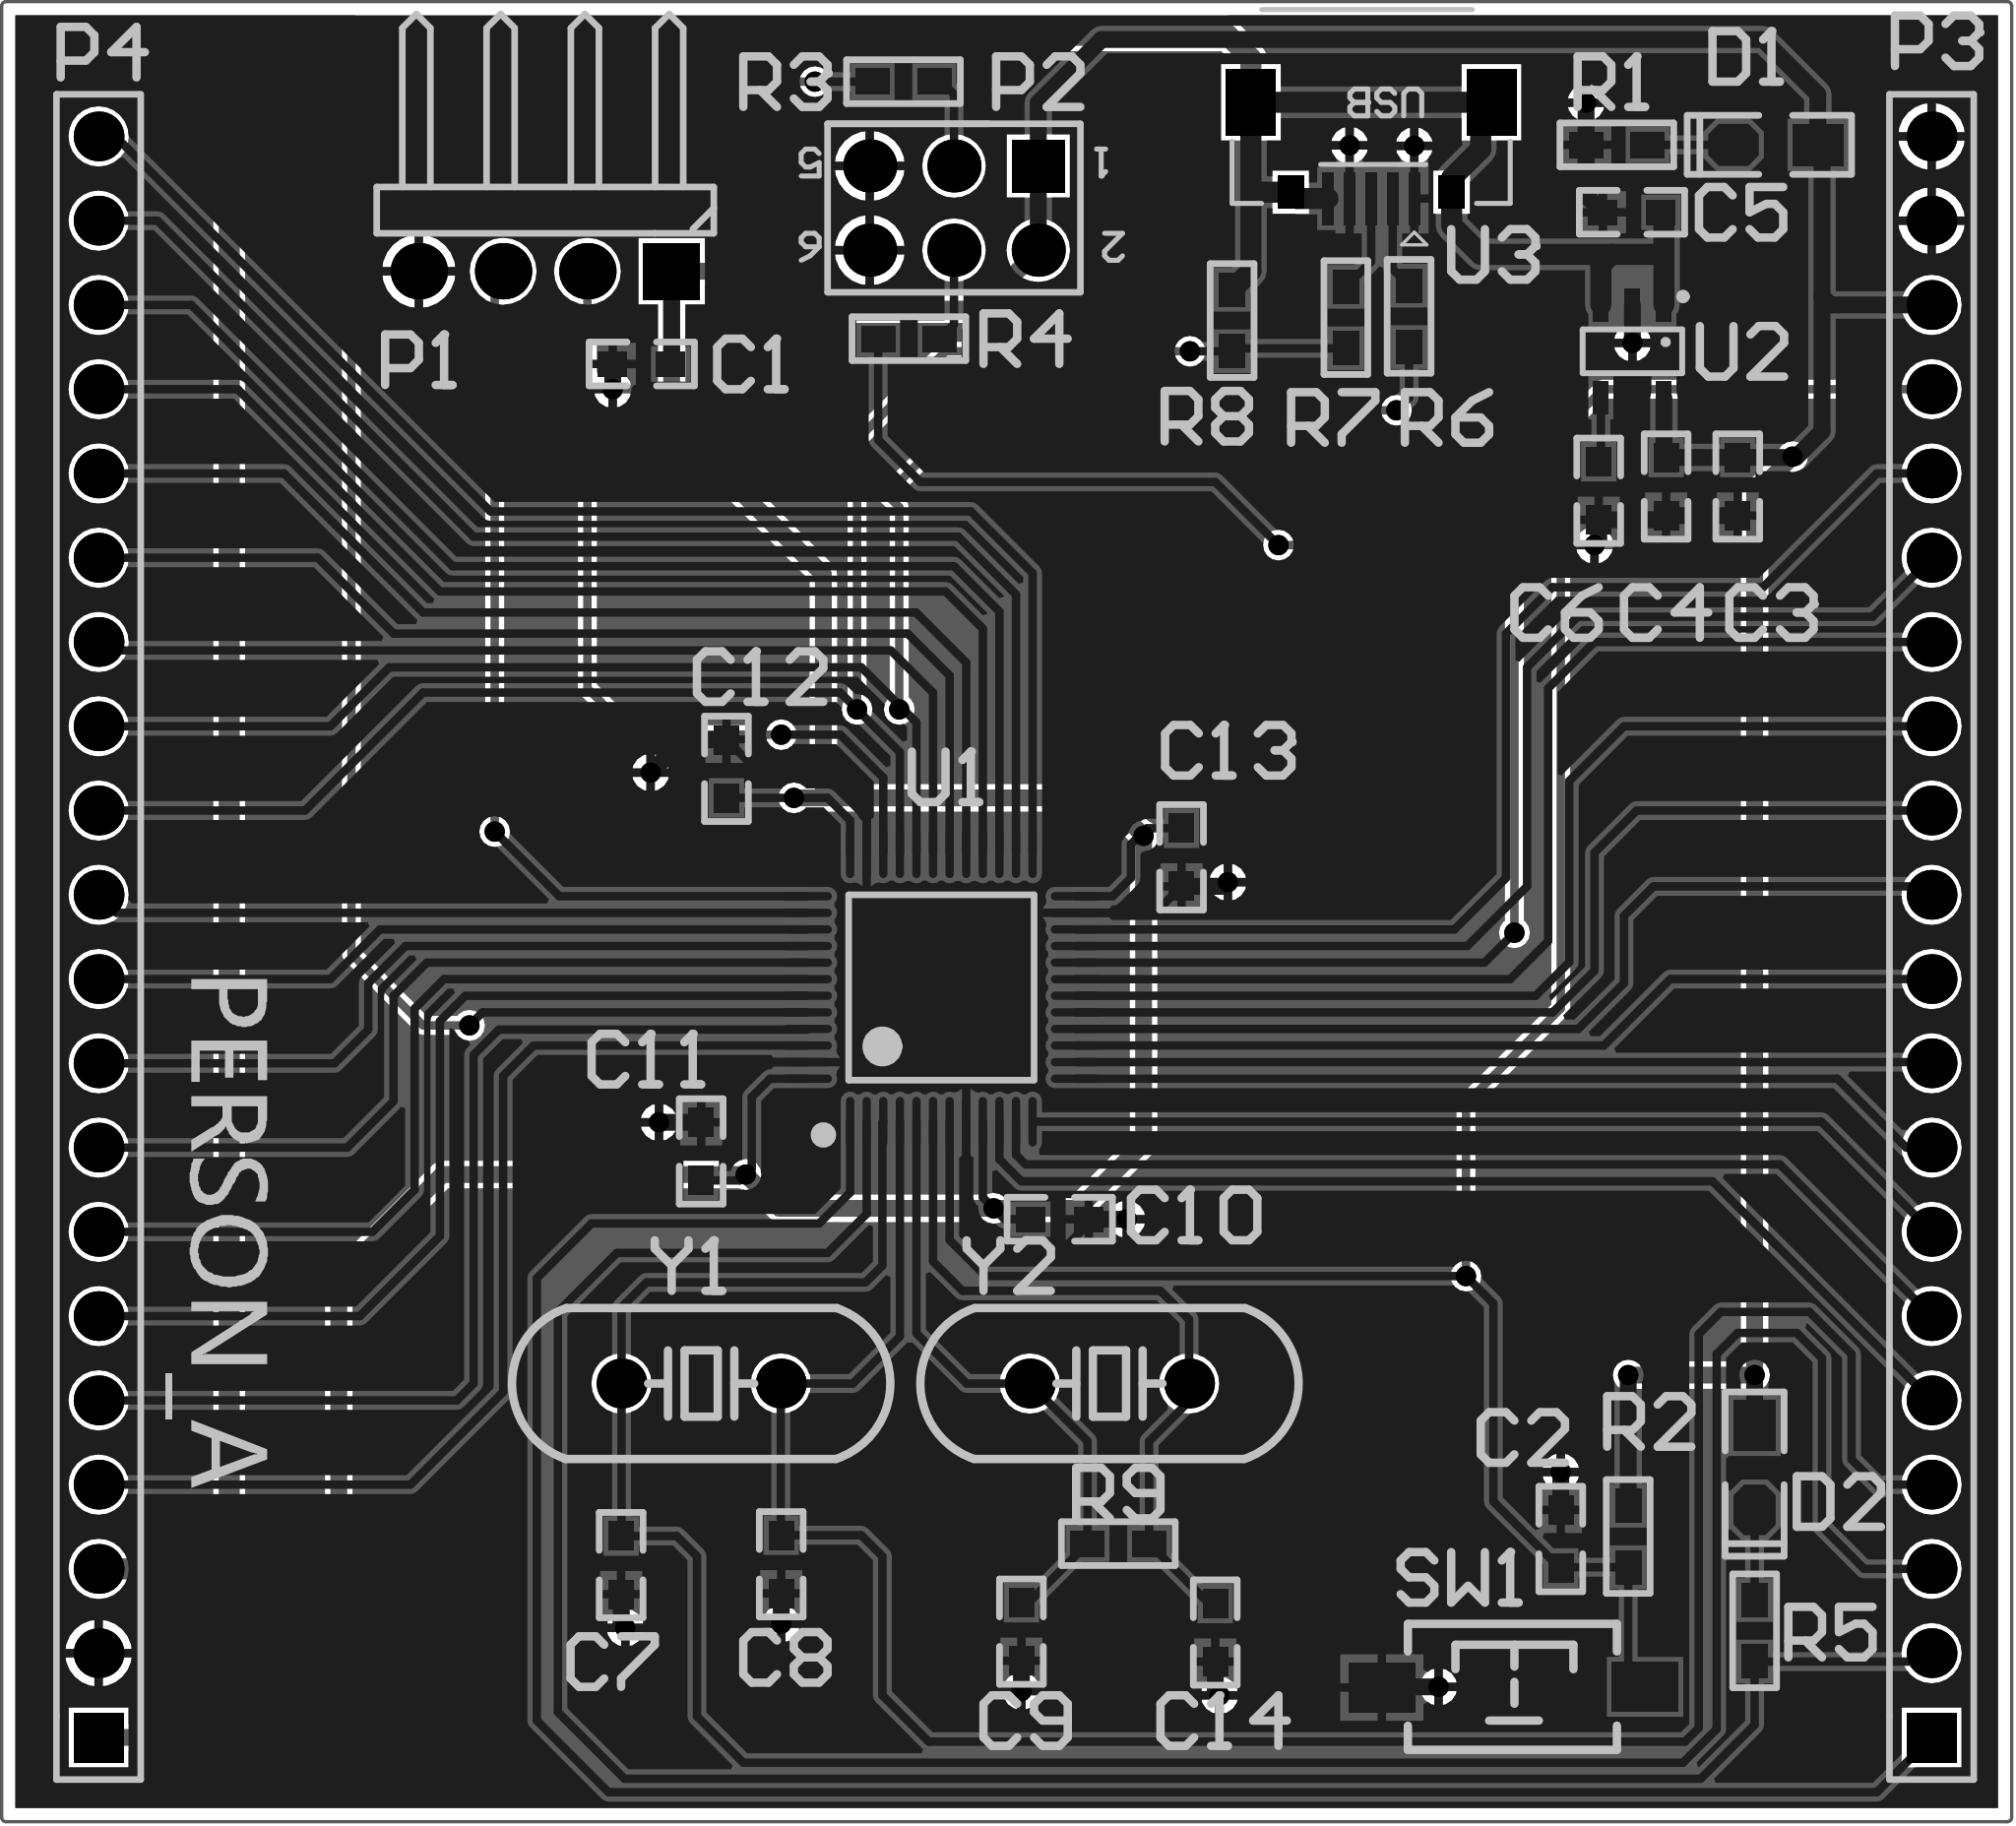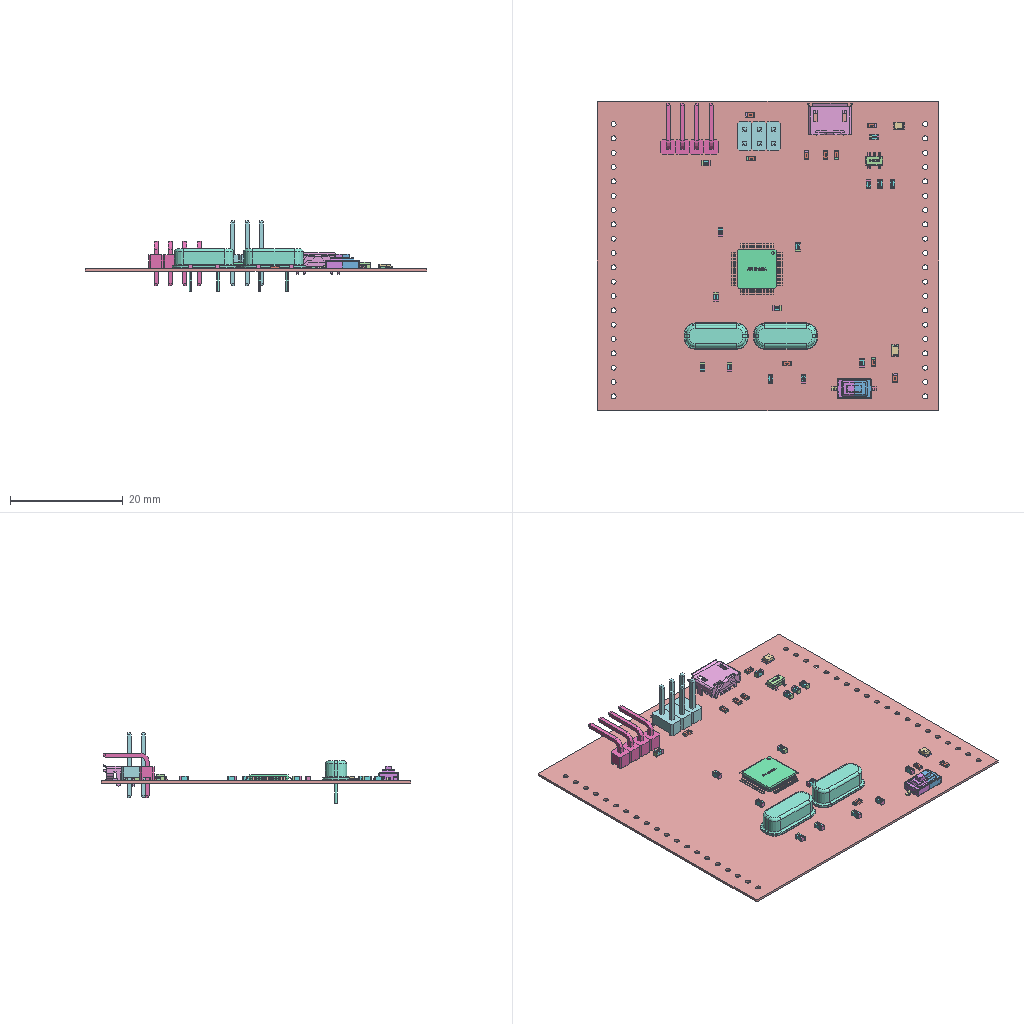Circuit board layout | Altium Designer | box 60.6 x 54.9 x 12.5 mm
Layer stack:
# Altium Designer layer stack of  (unit mm; dielectric type: 0 none, 1 core, 2 prepreg, 3 surface material)
index,name,kind,layer,copper_thickness_mm,dielectric_type,dielectric_thickness_mm,dielectric_material,dielectric_constant
0,Top Paste,other,,,,,,
1,Top Overlay,other,,,,,,
2,Top Solder,dielectric,,,3,0.0102,Solder Resist,3.5
3,Top Layer,copper,Top Layer,0.0356,,,,
4,Dielectric 1,dielectric,,,0,0.32,FR-4,4.8
5,Bottom Layer,copper,Bottom Layer,0.0356,,,,
6,Bottom Solder,dielectric,,,3,0.0102,Solder Resist,3.5
7,Bottom Overlay,other,,,,,,
8,Bottom Paste,other,,,,,,
# drill layer pairs: low layer,high layer
drill_pair,Top Layer,Bottom Layer
Part placement:
Designator,Comment,Layer,Footprint,Center-X(mm),Center-Y(mm),Rotation
C1,105 C0603,TopLayer,C_0603,84.569,116.205,0
C2,105 C0603,TopLayer,C_0603,112.268,80.785,270
C3,105 C0603,TopLayer,C_0603,117.602,112.509,90
C4,105 C0603,TopLayer,C_0603,115.443,112.509,90
C5,105 C0603,TopLayer,C_0603,114.414,120.777,0
C6,105 C0603,TopLayer,C_0603,113.411,112.382,90
C7,22P,0603,TopLayer,C_0603,83.947,79.997,270
C8,22P,0603,TopLayer,C_0603,88.773,80.023,270
C9,22P,0603,TopLayer,C_0603,96.012,77.991,270
C10,105 C0603,TopLayer,C_0603,97.168,90.424,180
C11,105 C0603,TopLayer,C_0603,86.36,92.469,270
C12,105 C0603,TopLayer,C_0603,87.122,104,270
C13,105 C0603,TopLayer,C_0603,100.838,101.333,90
C14,22P,0603,TopLayer,C_0603,101.854,77.965,270
D1,LED,TopLayer,LED_0805G,118.745,122.809,180
D2,LED,TopLayer,LED_0805G,118.11,82.931,270
P1,SWD,TopLayer,HDR-1X4_H,81.661,118.999,180
P2,Header 3X2,TopLayer,HDR-3X2,93.98,120.904,180
P3,Header 20,TopLayer,HDR1X20,123.444,98.933,90
P4,Header 20,TopLayer,HDR1X20,68.199,98.933,90
R1,10K R0603,TopLayer,R_0603,113.957,122.809,180
R3,10K R0603,TopLayer,R_0603,92.456,124.714,0
R4,10K R0603,TopLayer,R_0603,92.621,116.967,180
R5,10K R0603,TopLayer,R_0603,118.11,78.016,270
R6,20R,0603,TopLayer,R_0603,107.696,117.64,270
R7,20R0603,TopLayer,R_0603,105.791,117.602,270
R8,4.7K,0603,TopLayer,R_0603,102.362,117.513,270
R9,1M0603,TopLayer,R_0603,98.933,80.645,180
SW1,SW-PB_V,TopLayer,TSW_SMD-3*6*2.5,110.842,76.317,360
U1,stm32f103c8t6_48pin,TopLayer,TQFP48_7x7_L,93.599,97.409,0
U2,RT9193,TopLayer,SOT23-5L,114.427,116.586,180
U3,USB-mrico,TopLayer,USB-micro_B,106.553,122.642,180
Y1,32.768K,TopLayer,XTAL-49S_DIP,86.36,85.471,180
Y2,8M,TopLayer,XTAL-49S_DIP,98.666,85.471,180
R2,10K R0603,TopLayer,R_0603,114.3,80.861,90
Pad and via stacks:
# Altium Designer via and pad stacks of  (unit mm). Each distinct definition once, with the count of objects using it.
# via: kind,start_layer,end_layer,hole_mm,diameter_mm,mode(0 simple;1 top-mid-bottom;2 full stack),diameter_per_layer,count,example_net
# pad: kind,layer,hole_mm,hole_type(0 round;1 square;2 slot),plating,top_size,top_shape(1 round;2 rect;3 octagon;9 rounded rect),mid_size,bottom_size,mode,footprint,size_per_layer,count,example
pad,Top Layer,0,0,plated,0.889x0.762,2,0.889x0.762,0.889x0.762,0,C 0603,,28,C14.2
pad,Top Layer,0,0,plated,1.016x0.8,2,1.016x0.8,1.016x0.8,0,R 0603,,18,R9.1
pad,Top Layer,0,0,plated,1.6x0.35,2,1.6x0.35,1.6x0.35,0,USB-micro_B,,5,U3.2
pad,Top Layer,0,0,plated,0.45x1,2,0.45x1,0.45x1,0,SOT23-5L,,5,U2.4
pad,Top Layer,0,0,plated,0.25x1.5,1,0.25x1.5,0.25x1.5,0,TQFP48 7x7_L,,48,U1.1
pad,Top Layer,0,0,plated,2x1.5,2,2x1.5,2x1.5,0,TSW SMD-3*6*2.5,,2,SW1.1
pad,Top Layer,0,0,plated,1.524x1.27,2,1.524x1.27,1.524x1.27,0,LED 0805G,,2,D2.1
pad,Top Layer,0,0,plated,1.524x1.27,3,1.524x1.27,1.524x1.27,0,LED 0805G,,2,D2.2
pad,Multi-Layer,0.8,0,plated,1.5x1.5,1,1.5x1.5,1.5x1.5,0,XTAL-49S DIP,,4,Y2.2
pad,Multi-Layer,0.5,2,plated,1.5x2,2,1.5x2,1.5x2,0,USB-micro_B,,2,U3.5
pad,Multi-Layer,0.5,0,plated,0.8x1,2,0.8x1,0.8x1,0,USB-micro_B,,2,U3.5
pad,Multi-Layer,0.9,0,plated,1.5x1.5,2,1.5x1.5,1.5x1.5,0,HDR1X20,,2,P4.1
pad,Multi-Layer,0.9,0,plated,1.5x1.5,1,1.5x1.5,1.5x1.5,0,HDR1X20,,38,P4.2
pad,Multi-Layer,0.9,0,plated,1.6x1.6,2,1.6x1.6,1.6x1.6,0,HDR-3X2,,1,P2.1
pad,Multi-Layer,0.9,0,plated,1.6x1.6,1,1.6x1.6,1.6x1.6,0,HDR-3X2,,5,P2.2
pad,Multi-Layer,0.9,0,plated,1.7x1.7,2,1.7x1.7,1.7x1.7,0,HDR-1X4_H,,1,P1.1
pad,Multi-Layer,0.9,0,plated,1.7x1.7,1,1.7x1.7,1.7x1.7,0,HDR-1X4_H,,3,P1.2
via,Top Layer,Bottom Layer,0.3048,0.6096,0,,34,SWDCLK
Copper pours:
name,layer,net,type(0 solid;1 hatched;2 none)
D,Top Layer,GND,0
D,Bottom Layer,GND,0
Design rules, without the lines most boards share:
# Altium Designer design rules of  (exported by Altium Designer, unit mm)
# columns: name | kind | enabled | priority | scope1 | scope2 | descriptor | typed fields (field=value)
Clearance | 0 | enabled | 1 | All | All | Clearance Constraint (Gap=6mil) (All),(All) | gap=0.1524
PlaneConnect | 6 | enabled | 1 | All | All | Power Plane Connect Rule(Relief Connect )(Expansion=20mil) (Conductor Width=10mil) (Air Gap=10mil) (Entries=4) (All) | relief_conductor_width=0.254 relief_entries=4 relief_expansion=0.508
PolygonConnect | 20 | enabled | 1 | All | All | Polygon Connect Rule(Relief Connect )(Conductor Width=10mil) (Relief Angle=90 Angle) (Entries=4) (Air Gap Width=10mil) (All),(All) | connect_style(0=relief,1=direct,2=none)=0 relief_conductor_width=0.254 relief_entries=4
Width | 2 | enabled | 1 | All | All | Width Constraint (Min=10mil) (Max=30mil) (Preferred=10mil) (All) |
RoutingVias | 11 | enabled | 1 | All | All | Routing Via (MinHoleWidth=28mil) (MaxHoleWidth=28mil) (PreferredHoleWidth=28mil) (MinWidth=50mil) (MaxWidth=50mil) (PreferedWidth=50mil) (All) | via_min_hole=0.7112 via_max_hole=0.7112 via_preferred_diameter=1.27 via_preferred_hole=0.7112
PasteMaskExpansion | 14 | enabled | 1 | All | All | Paste Mask Expansion (Expansion =0mil) (All) | expansion=0
SolderMaskExpansion | 13 | enabled | 1 | All | All | Solder Mask Expansion (Expansion =4mil) (All) | expansion=0.1016
DiffPairsRouting | 51 | enabled | 1 | All | All | Differential Pairs Uncoupled Length using the Gap Constraints (Min=10mil) (Max=10mil) (Prefered=10mil)  and Width Constraints (Min=15mil) (Max=15mil) (Prefered=15mil) (All) |
HoleToHoleClearance | 52 | enabled | 1 | All | All | Hole To Hole Clearance (Gap=10mil) (All),(All) | gap=0.254
MinimumSolderMaskSliver | 53 | enabled | 1 | All | All | Minimum Solder Mask Sliver (Gap=0mil) (All),(All) |
SilkToSolderMaskClearance | 54 | enabled | 1 | IsPad | All | Silk To Solder Mask (Clearance=0mil) (IsPad),(All) |
SilkToSilkClearance | 55 | enabled | 1 | All | All | Silk to Silk (Clearance=0mil) (All),(All) |